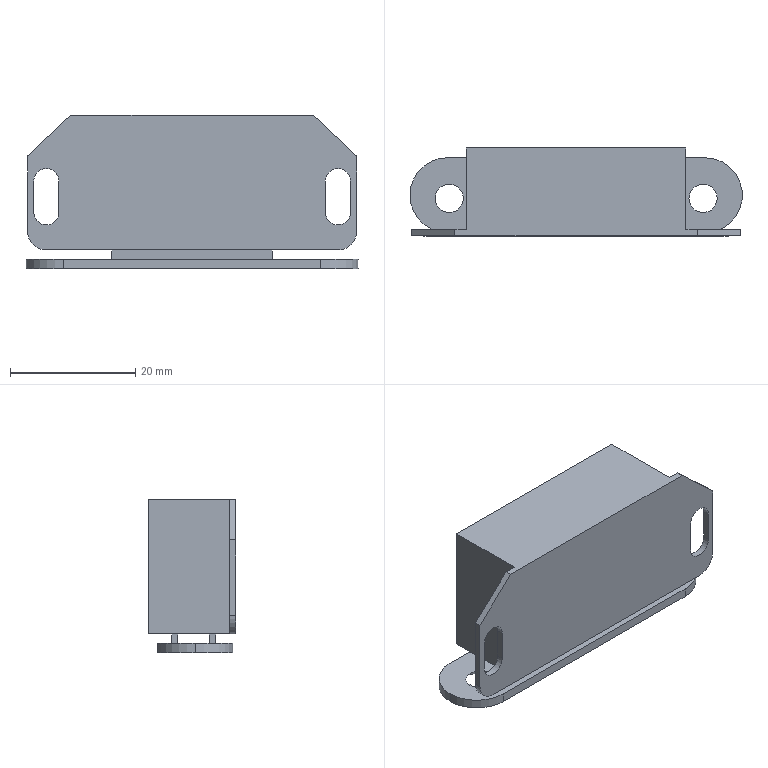Part | SolidWorks | features BaseBody 1 | 1 solid | 43 faces | box 53 x 14 x 24.5 mm | volume 11695 mm3 | plane 28 | cylinder 11 | cone 4 | commonest cylinder face diameters 4 x6 12 x3 6 x2
STEP:
#1=CARTESIAN_POINT('',(-21.25,0.,-10.5));
#2=VERTEX_POINT('',#1);
#3=CARTESIAN_POINT('',(-23.25,0.,-8.5));
#4=VERTEX_POINT('',#3);
#5=CARTESIAN_POINT('',(-23.25,0.,-10.5));
#6=DIRECTION('',(0.,-1.,0.));
#7=DIRECTION('',(0.,0.,1.));
#8=AXIS2_PLACEMENT_3D('',#5,#6,#7);
#9=CIRCLE('',#8,2.);
#10=EDGE_CURVE('',#2,#4,#9,.T.);
#11=ORIENTED_EDGE('',*,*,#10,.T.);
#12=CARTESIAN_POINT('',(-23.25,1.,-8.5));
#13=VERTEX_POINT('',#12);
#14=CARTESIAN_POINT('',(-23.25,1.,-8.5));
#15=DIRECTION('',(0.,1.,0.));
#16=VECTOR('',#15,1000.);
#17=LINE('',#14,#16);
#18=EDGE_CURVE('',#4,#13,#17,.T.);
#19=ORIENTED_EDGE('',*,*,#18,.T.);
#20=CARTESIAN_POINT('',(-21.25,1.,-10.5));
#21=VERTEX_POINT('',#20);
#22=CARTESIAN_POINT('',(-23.25,1.,-10.5));
#23=DIRECTION('',(0.,-1.,0.));
#24=DIRECTION('',(0.,0.,1.));
#25=AXIS2_PLACEMENT_3D('',#22,#23,#24);
#26=CIRCLE('',#25,2.);
#27=EDGE_CURVE('',#21,#13,#26,.T.);
#28=ORIENTED_EDGE('',*,*,#27,.F.);
#29=CARTESIAN_POINT('',(-21.25,1.,-10.5));
#30=DIRECTION('',(0.,1.,0.));
#31=VECTOR('',#30,1000.);
#32=LINE('',#29,#31);
#33=EDGE_CURVE('',#2,#21,#32,.T.);
#34=ORIENTED_EDGE('',*,*,#33,.F.);
#35=EDGE_LOOP('',(#11,#19,#28,#34));
#36=FACE_OUTER_BOUND('',#35,.T.);
#37=CARTESIAN_POINT('',(-23.25,1.,-10.5));
#38=DIRECTION('',(0.,1.,0.));
#39=DIRECTION('',(0.,0.,1.));
#40=AXIS2_PLACEMENT_3D('',#37,#38,#39);
#41=CYLINDRICAL_SURFACE('',#40,2.);
#42=ADVANCED_FACE('',(#36),#41,.F.);
#43=CARTESIAN_POINT('',(25.25,0.,-10.5));
#44=VERTEX_POINT('',#43);
#45=CARTESIAN_POINT('',(23.25,0.,-8.5));
#46=VERTEX_POINT('',#45);
#47=CARTESIAN_POINT('',(23.25,0.,-10.5));
#48=DIRECTION('',(0.,-1.,0.));
#49=DIRECTION('',(0.,0.,1.));
#50=AXIS2_PLACEMENT_3D('',#47,#48,#49);
#51=CIRCLE('',#50,2.);
#52=EDGE_CURVE('',#44,#46,#51,.T.);
#53=ORIENTED_EDGE('',*,*,#52,.T.);
#54=CARTESIAN_POINT('',(23.25,1.,-8.5));
#55=VERTEX_POINT('',#54);
#56=CARTESIAN_POINT('',(23.25,1.,-8.5));
#57=DIRECTION('',(0.,1.,0.));
#58=VECTOR('',#57,1000.);
#59=LINE('',#56,#58);
#60=EDGE_CURVE('',#46,#55,#59,.T.);
#61=ORIENTED_EDGE('',*,*,#60,.T.);
#62=CARTESIAN_POINT('',(25.25,1.,-10.5));
#63=VERTEX_POINT('',#62);
#64=CARTESIAN_POINT('',(23.25,1.,-10.5));
#65=DIRECTION('',(0.,-1.,0.));
#66=DIRECTION('',(0.,0.,1.));
#67=AXIS2_PLACEMENT_3D('',#64,#65,#66);
#68=CIRCLE('',#67,2.);
#69=EDGE_CURVE('',#63,#55,#68,.T.);
#70=ORIENTED_EDGE('',*,*,#69,.F.);
#71=CARTESIAN_POINT('',(25.25,1.,-10.5));
#72=DIRECTION('',(0.,1.,0.));
#73=VECTOR('',#72,1000.);
#74=LINE('',#71,#73);
#75=EDGE_CURVE('',#44,#63,#74,.T.);
#76=ORIENTED_EDGE('',*,*,#75,.F.);
#77=EDGE_LOOP('',(#53,#61,#70,#76));
#78=FACE_OUTER_BOUND('',#77,.T.);
#79=CARTESIAN_POINT('',(23.25,1.,-10.5));
#80=DIRECTION('',(0.,1.,0.));
#81=DIRECTION('',(0.,0.,1.));
#82=AXIS2_PLACEMENT_3D('',#79,#80,#81);
#83=CYLINDRICAL_SURFACE('',#82,2.);
#84=ADVANCED_FACE('',(#78),#83,.F.);
#85=CARTESIAN_POINT('',(-26.5,6.5,-23.));
#86=VERTEX_POINT('',#85);
#87=CARTESIAN_POINT('',(-20.5,0.5,-23.));
#88=VERTEX_POINT('',#87);
#89=CARTESIAN_POINT('',(-20.5,6.5,-23.));
#90=DIRECTION('',(0.,0.,1.));
#91=DIRECTION('',(-1.,0.,0.));
#92=AXIS2_PLACEMENT_3D('',#89,#90,#91);
#93=CIRCLE('',#92,6.);
#94=EDGE_CURVE('',#86,#88,#93,.T.);
#95=ORIENTED_EDGE('',*,*,#94,.F.);
#96=CARTESIAN_POINT('',(-26.5,6.5,-24.5));
#97=VERTEX_POINT('',#96);
#98=CARTESIAN_POINT('',(-26.5,6.5,-24.5));
#99=DIRECTION('',(0.,0.,-1.));
#100=VECTOR('',#99,1000.);
#101=LINE('',#98,#100);
#102=EDGE_CURVE('',#86,#97,#101,.T.);
#103=ORIENTED_EDGE('',*,*,#102,.T.);
#104=CARTESIAN_POINT('',(-20.5,0.5,-24.5));
#105=VERTEX_POINT('',#104);
#106=CARTESIAN_POINT('',(-20.5,6.5,-24.5));
#107=DIRECTION('',(0.,0.,1.));
#108=DIRECTION('',(-1.,0.,0.));
#109=AXIS2_PLACEMENT_3D('',#106,#107,#108);
#110=CIRCLE('',#109,6.);
#111=EDGE_CURVE('',#97,#105,#110,.T.);
#112=ORIENTED_EDGE('',*,*,#111,.T.);
#113=CARTESIAN_POINT('',(-20.5,0.5,-24.5));
#114=DIRECTION('',(0.,0.,-1.));
#115=VECTOR('',#114,1000.);
#116=LINE('',#113,#115);
#117=EDGE_CURVE('',#88,#105,#116,.T.);
#118=ORIENTED_EDGE('',*,*,#117,.F.);
#119=EDGE_LOOP('',(#95,#103,#112,#118));
#120=FACE_OUTER_BOUND('',#119,.T.);
#121=CARTESIAN_POINT('',(-20.5,6.5,-24.5));
#122=DIRECTION('',(0.,0.,-1.));
#123=DIRECTION('',(-1.,0.,0.));
#124=AXIS2_PLACEMENT_3D('',#121,#122,#123);
#125=CYLINDRICAL_SURFACE('',#124,6.);
#126=ADVANCED_FACE('',(#120),#125,.T.);
#127=CARTESIAN_POINT('',(-18.,6.,-23.));
#128=VERTEX_POINT('',#127);
#129=CARTESIAN_POINT('',(-22.5,6.,-23.));
#130=VERTEX_POINT('',#129);
#131=CARTESIAN_POINT('',(-20.25,6.,-23.));
#132=DIRECTION('',(0.,0.,-1.));
#133=DIRECTION('',(-1.,0.,0.));
#134=AXIS2_PLACEMENT_3D('',#131,#132,#133);
#135=CIRCLE('',#134,2.25);
#136=EDGE_CURVE('',#128,#130,#135,.T.);
#137=ORIENTED_EDGE('',*,*,#136,.F.);
#138=CARTESIAN_POINT('',(-16.5,6.,-24.5));
#139=VERTEX_POINT('',#138);
#140=CARTESIAN_POINT('',(-16.5,6.,-24.5));
#141=DIRECTION('',(0.7071,0.,-0.7071));
#142=VECTOR('',#141,1000.);
#143=LINE('',#140,#142);
#144=EDGE_CURVE('',#128,#139,#143,.T.);
#145=ORIENTED_EDGE('',*,*,#144,.T.);
#146=CARTESIAN_POINT('',(-24.,6.,-24.5));
#147=VERTEX_POINT('',#146);
#148=CARTESIAN_POINT('',(-20.25,6.,-24.5));
#149=DIRECTION('',(0.,0.,1.));
#150=DIRECTION('',(-1.,0.,0.));
#151=AXIS2_PLACEMENT_3D('',#148,#149,#150);
#152=CIRCLE('',#151,3.75);
#153=EDGE_CURVE('',#147,#139,#152,.T.);
#154=ORIENTED_EDGE('',*,*,#153,.F.);
#155=CARTESIAN_POINT('',(-24.,6.,-24.5));
#156=DIRECTION('',(-0.7071,0.,-0.7071));
#157=VECTOR('',#156,1000.);
#158=LINE('',#155,#157);
#159=EDGE_CURVE('',#130,#147,#158,.T.);
#160=ORIENTED_EDGE('',*,*,#159,.F.);
#161=EDGE_LOOP('',(#137,#145,#154,#160));
#162=FACE_OUTER_BOUND('',#161,.T.);
#163=CARTESIAN_POINT('',(-20.25,6.,-24.5));
#164=DIRECTION('',(0.,0.,-1.));
#165=DIRECTION('',(-1.,0.,0.));
#166=AXIS2_PLACEMENT_3D('',#163,#164,#165);
#167=CONICAL_SURFACE('',#166,3.75,0.7854);
#168=ADVANCED_FACE('',(#162),#167,.F.);
#169=CARTESIAN_POINT('',(22.5,6.,-23.));
#170=VERTEX_POINT('',#169);
#171=CARTESIAN_POINT('',(18.,6.,-23.));
#172=VERTEX_POINT('',#171);
#173=CARTESIAN_POINT('',(20.25,6.,-23.));
#174=DIRECTION('',(0.,0.,-1.));
#175=DIRECTION('',(-1.,0.,0.));
#176=AXIS2_PLACEMENT_3D('',#173,#174,#175);
#177=CIRCLE('',#176,2.25);
#178=EDGE_CURVE('',#170,#172,#177,.T.);
#179=ORIENTED_EDGE('',*,*,#178,.F.);
#180=CARTESIAN_POINT('',(24.,6.,-24.5));
#181=VERTEX_POINT('',#180);
#182=CARTESIAN_POINT('',(24.,6.,-24.5));
#183=DIRECTION('',(0.7071,0.,-0.7071));
#184=VECTOR('',#183,1000.);
#185=LINE('',#182,#184);
#186=EDGE_CURVE('',#170,#181,#185,.T.);
#187=ORIENTED_EDGE('',*,*,#186,.T.);
#188=CARTESIAN_POINT('',(16.5,6.,-24.5));
#189=VERTEX_POINT('',#188);
#190=CARTESIAN_POINT('',(20.25,6.,-24.5));
#191=DIRECTION('',(0.,0.,1.));
#192=DIRECTION('',(-1.,0.,0.));
#193=AXIS2_PLACEMENT_3D('',#190,#191,#192);
#194=CIRCLE('',#193,3.75);
#195=EDGE_CURVE('',#189,#181,#194,.T.);
#196=ORIENTED_EDGE('',*,*,#195,.F.);
#197=CARTESIAN_POINT('',(16.5,6.,-24.5));
#198=DIRECTION('',(-0.7071,0.,-0.7071));
#199=VECTOR('',#198,1000.);
#200=LINE('',#197,#199);
#201=EDGE_CURVE('',#172,#189,#200,.T.);
#202=ORIENTED_EDGE('',*,*,#201,.F.);
#203=EDGE_LOOP('',(#179,#187,#196,#202));
#204=FACE_OUTER_BOUND('',#203,.T.);
#205=CARTESIAN_POINT('',(20.25,6.,-24.5));
#206=DIRECTION('',(0.,0.,-1.));
#207=DIRECTION('',(-1.,0.,0.));
#208=AXIS2_PLACEMENT_3D('',#205,#206,#207);
#209=CONICAL_SURFACE('',#208,3.75,0.7854);
#210=ADVANCED_FACE('',(#204),#209,.F.);
#211=ORIENTED_EDGE('',*,*,#10,.F.);
#212=CARTESIAN_POINT('',(-21.25,0.,-15.5));
#213=VERTEX_POINT('',#212);
#214=CARTESIAN_POINT('',(-21.25,0.,-18.5));
#215=DIRECTION('',(0.,0.,1.));
#216=VECTOR('',#215,1000.);
#217=LINE('',#214,#216);
#218=EDGE_CURVE('',#213,#2,#217,.T.);
#219=ORIENTED_EDGE('',*,*,#218,.F.);
#220=CARTESIAN_POINT('',(-25.25,0.,-15.5));
#221=VERTEX_POINT('',#220);
#222=CARTESIAN_POINT('',(-23.25,0.,-15.5));
#223=DIRECTION('',(0.,-1.,0.));
#224=DIRECTION('',(0.,0.,1.));
#225=AXIS2_PLACEMENT_3D('',#222,#223,#224);
#226=CIRCLE('',#225,2.);
#227=EDGE_CURVE('',#221,#213,#226,.T.);
#228=ORIENTED_EDGE('',*,*,#227,.F.);
#229=CARTESIAN_POINT('',(-25.25,0.,-10.5));
#230=VERTEX_POINT('',#229);
#231=CARTESIAN_POINT('',(-25.25,0.,-18.5));
#232=DIRECTION('',(0.,0.,-1.));
#233=VECTOR('',#232,1000.);
#234=LINE('',#231,#233);
#235=EDGE_CURVE('',#230,#221,#234,.T.);
#236=ORIENTED_EDGE('',*,*,#235,.F.);
#237=CARTESIAN_POINT('',(-23.25,0.,-10.5));
#238=DIRECTION('',(0.,-1.,0.));
#239=DIRECTION('',(0.,0.,1.));
#240=AXIS2_PLACEMENT_3D('',#237,#238,#239);
#241=CIRCLE('',#240,2.);
#242=EDGE_CURVE('',#4,#230,#241,.T.);
#243=ORIENTED_EDGE('',*,*,#242,.F.);
#244=EDGE_LOOP('',(#211,#219,#228,#236,#243));
#245=FACE_BOUND('',#244,.T.);
#246=ORIENTED_EDGE('',*,*,#52,.F.);
#247=CARTESIAN_POINT('',(25.25,0.,-15.5));
#248=VERTEX_POINT('',#247);
#249=CARTESIAN_POINT('',(25.25,0.,-18.5));
#250=DIRECTION('',(0.,0.,1.));
#251=VECTOR('',#250,1000.);
#252=LINE('',#249,#251);
#253=EDGE_CURVE('',#248,#44,#252,.T.);
#254=ORIENTED_EDGE('',*,*,#253,.F.);
#255=CARTESIAN_POINT('',(21.25,0.,-15.5));
#256=VERTEX_POINT('',#255);
#257=CARTESIAN_POINT('',(23.25,0.,-15.5));
#258=DIRECTION('',(0.,-1.,0.));
#259=DIRECTION('',(0.,0.,1.));
#260=AXIS2_PLACEMENT_3D('',#257,#258,#259);
#261=CIRCLE('',#260,2.);
#262=EDGE_CURVE('',#256,#248,#261,.T.);
#263=ORIENTED_EDGE('',*,*,#262,.F.);
#264=CARTESIAN_POINT('',(21.25,0.,-10.5));
#265=VERTEX_POINT('',#264);
#266=CARTESIAN_POINT('',(21.25,0.,-18.5));
#267=DIRECTION('',(0.,0.,-1.));
#268=VECTOR('',#267,1000.);
#269=LINE('',#266,#268);
#270=EDGE_CURVE('',#265,#256,#269,.T.);
#271=ORIENTED_EDGE('',*,*,#270,.F.);
#272=CARTESIAN_POINT('',(23.25,0.,-10.5));
#273=DIRECTION('',(0.,-1.,0.));
#274=DIRECTION('',(0.,0.,1.));
#275=AXIS2_PLACEMENT_3D('',#272,#273,#274);
#276=CIRCLE('',#275,2.);
#277=EDGE_CURVE('',#46,#265,#276,.T.);
#278=ORIENTED_EDGE('',*,*,#277,.F.);
#279=EDGE_LOOP('',(#246,#254,#263,#271,#278));
#280=FACE_BOUND('',#279,.T.);
#281=CARTESIAN_POINT('',(-19.344,0.,0.));
#282=VERTEX_POINT('',#281);
#283=CARTESIAN_POINT('',(19.344,0.,0.));
#284=VERTEX_POINT('',#283);
#285=CARTESIAN_POINT('',(23.25,0.,0.));
#286=DIRECTION('',(1.,0.,0.));
#287=VECTOR('',#286,1000.);
#288=LINE('',#285,#287);
#289=EDGE_CURVE('',#282,#284,#288,.T.);
#290=ORIENTED_EDGE('',*,*,#289,.F.);
#291=CARTESIAN_POINT('',(-26.25,0.,-6.5));
#292=VERTEX_POINT('',#291);
#293=CARTESIAN_POINT('',(-26.25,0.,-6.5));
#294=DIRECTION('',(0.7282,0.,0.6854));
#295=VECTOR('',#294,1000.);
#296=LINE('',#293,#295);
#297=EDGE_CURVE('',#292,#282,#296,.T.);
#298=ORIENTED_EDGE('',*,*,#297,.F.);
#299=CARTESIAN_POINT('',(-26.25,0.,-18.5));
#300=VERTEX_POINT('',#299);
#301=CARTESIAN_POINT('',(-26.25,0.,-18.5));
#302=DIRECTION('',(0.,0.,1.));
#303=VECTOR('',#302,1000.);
#304=LINE('',#301,#303);
#305=EDGE_CURVE('',#300,#292,#304,.T.);
#306=ORIENTED_EDGE('',*,*,#305,.F.);
#307=CARTESIAN_POINT('',(-23.25,0.,-21.5));
#308=VERTEX_POINT('',#307);
#309=CARTESIAN_POINT('',(-23.25,0.,-18.5));
#310=DIRECTION('',(0.,1.,0.));
#311=DIRECTION('',(0.,0.,1.));
#312=AXIS2_PLACEMENT_3D('',#309,#310,#311);
#313=CIRCLE('',#312,3.);
#314=EDGE_CURVE('',#308,#300,#313,.T.);
#315=ORIENTED_EDGE('',*,*,#314,.F.);
#316=CARTESIAN_POINT('',(23.25,0.,-21.5));
#317=VERTEX_POINT('',#316);
#318=CARTESIAN_POINT('',(23.25,0.,-21.5));
#319=DIRECTION('',(-1.,0.,0.));
#320=VECTOR('',#319,1000.);
#321=LINE('',#318,#320);
#322=EDGE_CURVE('',#317,#308,#321,.T.);
#323=ORIENTED_EDGE('',*,*,#322,.F.);
#324=CARTESIAN_POINT('',(26.25,0.,-18.5));
#325=VERTEX_POINT('',#324);
#326=CARTESIAN_POINT('',(23.25,0.,-18.5));
#327=DIRECTION('',(0.,1.,0.));
#328=DIRECTION('',(0.,0.,1.));
#329=AXIS2_PLACEMENT_3D('',#326,#327,#328);
#330=CIRCLE('',#329,3.);
#331=EDGE_CURVE('',#325,#317,#330,.T.);
#332=ORIENTED_EDGE('',*,*,#331,.F.);
#333=CARTESIAN_POINT('',(26.25,0.,-6.5));
#334=VERTEX_POINT('',#333);
#335=CARTESIAN_POINT('',(26.25,0.,-18.5));
#336=DIRECTION('',(0.,0.,-1.));
#337=VECTOR('',#336,1000.);
#338=LINE('',#335,#337);
#339=EDGE_CURVE('',#334,#325,#338,.T.);
#340=ORIENTED_EDGE('',*,*,#339,.F.);
#341=CARTESIAN_POINT('',(19.344,0.,0.));
#342=DIRECTION('',(0.7282,0.,-0.6854));
#343=VECTOR('',#342,1000.);
#344=LINE('',#341,#343);
#345=EDGE_CURVE('',#284,#334,#344,.T.);
#346=ORIENTED_EDGE('',*,*,#345,.F.);
#347=EDGE_LOOP('',(#290,#298,#306,#315,#323,#332,#340,#346));
#348=FACE_OUTER_BOUND('',#347,.T.);
#349=CARTESIAN_POINT('',(23.25,0.,-18.5));
#350=DIRECTION('',(0.,1.,0.));
#351=DIRECTION('',(0.,0.,1.));
#352=AXIS2_PLACEMENT_3D('',#349,#350,#351);
#353=PLANE('',#352);
#354=ADVANCED_FACE('',(#245,#280,#348),#353,.F.);
#355=CARTESIAN_POINT('',(-25.25,1.,-15.5));
#356=VERTEX_POINT('',#355);
#357=CARTESIAN_POINT('',(-25.25,1.,-10.5));
#358=VERTEX_POINT('',#357);
#359=CARTESIAN_POINT('',(-25.25,1.,-15.5));
#360=DIRECTION('',(0.,0.,1.));
#361=VECTOR('',#360,1000.);
#362=LINE('',#359,#361);
#363=EDGE_CURVE('',#356,#358,#362,.T.);
#364=ORIENTED_EDGE('',*,*,#363,.T.);
#365=CARTESIAN_POINT('',(-25.25,1.,-10.5));
#366=DIRECTION('',(0.,-1.,0.));
#367=VECTOR('',#366,1000.);
#368=LINE('',#365,#367);
#369=EDGE_CURVE('',#358,#230,#368,.T.);
#370=ORIENTED_EDGE('',*,*,#369,.T.);
#371=ORIENTED_EDGE('',*,*,#235,.T.);
#372=CARTESIAN_POINT('',(-25.25,1.,-15.5));
#373=DIRECTION('',(0.,1.,0.));
#374=VECTOR('',#373,1000.);
#375=LINE('',#372,#374);
#376=EDGE_CURVE('',#221,#356,#375,.T.);
#377=ORIENTED_EDGE('',*,*,#376,.T.);
#378=EDGE_LOOP('',(#364,#370,#371,#377));
#379=FACE_OUTER_BOUND('',#378,.T.);
#380=CARTESIAN_POINT('',(-25.25,1.,-15.5));
#381=DIRECTION('',(1.,0.,0.));
#382=DIRECTION('',(0.,0.,-1.));
#383=AXIS2_PLACEMENT_3D('',#380,#381,#382);
#384=PLANE('',#383);
#385=ADVANCED_FACE('',(#379),#384,.T.);
#386=ORIENTED_EDGE('',*,*,#18,.F.);
#387=ORIENTED_EDGE('',*,*,#242,.T.);
#388=ORIENTED_EDGE('',*,*,#369,.F.);
#389=CARTESIAN_POINT('',(-23.25,1.,-10.5));
#390=DIRECTION('',(0.,-1.,0.));
#391=DIRECTION('',(0.,0.,1.));
#392=AXIS2_PLACEMENT_3D('',#389,#390,#391);
#393=CIRCLE('',#392,2.);
#394=EDGE_CURVE('',#13,#358,#393,.T.);
#395=ORIENTED_EDGE('',*,*,#394,.F.);
#396=EDGE_LOOP('',(#386,#387,#388,#395));
#397=FACE_OUTER_BOUND('',#396,.T.);
#398=CARTESIAN_POINT('',(-23.25,1.,-10.5));
#399=DIRECTION('',(0.,1.,0.));
#400=DIRECTION('',(0.,0.,1.));
#401=AXIS2_PLACEMENT_3D('',#398,#399,#400);
#402=CYLINDRICAL_SURFACE('',#401,2.);
#403=ADVANCED_FACE('',(#397),#402,.F.);
#404=CARTESIAN_POINT('',(-21.25,1.,-15.5));
#405=VERTEX_POINT('',#404);
#406=CARTESIAN_POINT('',(-21.25,1.,-10.5));
#407=DIRECTION('',(0.,0.,-1.));
#408=VECTOR('',#407,1000.);
#409=LINE('',#406,#408);
#410=EDGE_CURVE('',#21,#405,#409,.T.);
#411=ORIENTED_EDGE('',*,*,#410,.T.);
#412=CARTESIAN_POINT('',(-21.25,1.,-15.5));
#413=DIRECTION('',(0.,-1.,0.));
#414=VECTOR('',#413,1000.);
#415=LINE('',#412,#414);
#416=EDGE_CURVE('',#405,#213,#415,.T.);
#417=ORIENTED_EDGE('',*,*,#416,.T.);
#418=ORIENTED_EDGE('',*,*,#218,.T.);
#419=ORIENTED_EDGE('',*,*,#33,.T.);
#420=EDGE_LOOP('',(#411,#417,#418,#419));
#421=FACE_OUTER_BOUND('',#420,.T.);
#422=CARTESIAN_POINT('',(-21.25,1.,-10.5));
#423=DIRECTION('',(-1.,0.,0.));
#424=DIRECTION('',(0.,0.,1.));
#425=AXIS2_PLACEMENT_3D('',#422,#423,#424);
#426=PLANE('',#425);
#427=ADVANCED_FACE('',(#421),#426,.T.);
#428=ORIENTED_EDGE('',*,*,#416,.F.);
#429=CARTESIAN_POINT('',(-23.25,1.,-15.5));
#430=DIRECTION('',(0.,-1.,0.));
#431=DIRECTION('',(0.,0.,1.));
#432=AXIS2_PLACEMENT_3D('',#429,#430,#431);
#433=CIRCLE('',#432,2.);
#434=EDGE_CURVE('',#356,#405,#433,.T.);
#435=ORIENTED_EDGE('',*,*,#434,.F.);
#436=ORIENTED_EDGE('',*,*,#376,.F.);
#437=ORIENTED_EDGE('',*,*,#227,.T.);
#438=EDGE_LOOP('',(#428,#435,#436,#437));
#439=FACE_OUTER_BOUND('',#438,.T.);
#440=CARTESIAN_POINT('',(-23.25,1.,-15.5));
#441=DIRECTION('',(0.,1.,0.));
#442=DIRECTION('',(0.,0.,1.));
#443=AXIS2_PLACEMENT_3D('',#440,#441,#442);
#444=CYLINDRICAL_SURFACE('',#443,2.);
#445=ADVANCED_FACE('',(#439),#444,.F.);
#446=CARTESIAN_POINT('',(21.25,1.,-15.5));
#447=VERTEX_POINT('',#446);
#448=CARTESIAN_POINT('',(21.25,1.,-10.5));
#449=VERTEX_POINT('',#448);
#450=CARTESIAN_POINT('',(21.25,1.,-15.5));
#451=DIRECTION('',(0.,0.,1.));
#452=VECTOR('',#451,1000.);
#453=LINE('',#450,#452);
#454=EDGE_CURVE('',#447,#449,#453,.T.);
#455=ORIENTED_EDGE('',*,*,#454,.T.);
#456=CARTESIAN_POINT('',(21.25,1.,-10.5));
#457=DIRECTION('',(0.,-1.,0.));
#458=VECTOR('',#457,1000.);
#459=LINE('',#456,#458);
#460=EDGE_CURVE('',#449,#265,#459,.T.);
#461=ORIENTED_EDGE('',*,*,#460,.T.);
#462=ORIENTED_EDGE('',*,*,#270,.T.);
#463=CARTESIAN_POINT('',(21.25,1.,-15.5));
#464=DIRECTION('',(0.,1.,0.));
#465=VECTOR('',#464,1000.);
#466=LINE('',#463,#465);
#467=EDGE_CURVE('',#256,#447,#466,.T.);
#468=ORIENTED_EDGE('',*,*,#467,.T.);
#469=EDGE_LOOP('',(#455,#461,#462,#468));
#470=FACE_OUTER_BOUND('',#469,.T.);
#471=CARTESIAN_POINT('',(21.25,1.,-15.5));
#472=DIRECTION('',(1.,0.,0.));
#473=DIRECTION('',(0.,0.,-1.));
#474=AXIS2_PLACEMENT_3D('',#471,#472,#473);
#475=PLANE('',#474);
#476=ADVANCED_FACE('',(#470),#475,.T.);
#477=ORIENTED_EDGE('',*,*,#60,.F.);
#478=ORIENTED_EDGE('',*,*,#277,.T.);
#479=ORIENTED_EDGE('',*,*,#460,.F.);
#480=CARTESIAN_POINT('',(23.25,1.,-10.5));
#481=DIRECTION('',(0.,-1.,0.));
#482=DIRECTION('',(0.,0.,1.));
#483=AXIS2_PLACEMENT_3D('',#480,#481,#482);
#484=CIRCLE('',#483,2.);
#485=EDGE_CURVE('',#55,#449,#484,.T.);
#486=ORIENTED_EDGE('',*,*,#485,.F.);
#487=EDGE_LOOP('',(#477,#478,#479,#486));
#488=FACE_OUTER_BOUND('',#487,.T.);
#489=CARTESIAN_POINT('',(23.25,1.,-10.5));
#490=DIRECTION('',(0.,1.,0.));
#491=DIRECTION('',(0.,0.,1.));
#492=AXIS2_PLACEMENT_3D('',#489,#490,#491);
#493=CYLINDRICAL_SURFACE('',#492,2.);
#494=ADVANCED_FACE('',(#488),#493,.F.);
#495=CARTESIAN_POINT('',(25.25,1.,-15.5));
#496=VERTEX_POINT('',#495);
#497=CARTESIAN_POINT('',(25.25,1.,-10.5));
#498=DIRECTION('',(0.,0.,-1.));
#499=VECTOR('',#498,1000.);
#500=LINE('',#497,#499);
#501=EDGE_CURVE('',#63,#496,#500,.T.);
#502=ORIENTED_EDGE('',*,*,#501,.T.);
#503=CARTESIAN_POINT('',(25.25,1.,-15.5));
#504=DIRECTION('',(0.,-1.,0.));
#505=VECTOR('',#504,1000.);
#506=LINE('',#503,#505);
#507=EDGE_CURVE('',#496,#248,#506,.T.);
#508=ORIENTED_EDGE('',*,*,#507,.T.);
#509=ORIENTED_EDGE('',*,*,#253,.T.);
#510=ORIENTED_EDGE('',*,*,#75,.T.);
#511=EDGE_LOOP('',(#502,#508,#509,#510));
#512=FACE_OUTER_BOUND('',#511,.T.);
#513=CARTESIAN_POINT('',(25.25,1.,-10.5));
#514=DIRECTION('',(-1.,0.,0.));
#515=DIRECTION('',(0.,0.,1.));
#516=AXIS2_PLACEMENT_3D('',#513,#514,#515);
#517=PLANE('',#516);
#518=ADVANCED_FACE('',(#512),#517,.T.);
#519=ORIENTED_EDGE('',*,*,#507,.F.);
#520=CARTESIAN_POINT('',(23.25,1.,-15.5));
#521=DIRECTION('',(0.,-1.,0.));
#522=DIRECTION('',(0.,0.,1.));
#523=AXIS2_PLACEMENT_3D('',#520,#521,#522);
#524=CIRCLE('',#523,2.);
#525=EDGE_CURVE('',#447,#496,#524,.T.);
#526=ORIENTED_EDGE('',*,*,#525,.F.);
#527=ORIENTED_EDGE('',*,*,#467,.F.);
#528=ORIENTED_EDGE('',*,*,#262,.T.);
#529=EDGE_LOOP('',(#519,#526,#527,#528));
#530=FACE_OUTER_BOUND('',#529,.T.);
#531=CARTESIAN_POINT('',(23.25,1.,-15.5));
#532=DIRECTION('',(0.,1.,0.));
#533=DIRECTION('',(0.,0.,1.));
#534=AXIS2_PLACEMENT_3D('',#531,#532,#533);
#535=CYLINDRICAL_SURFACE('',#534,2.);
#536=ADVANCED_FACE('',(#530),#535,.F.);
#537=CARTESIAN_POINT('',(26.25,1.,-6.5));
#538=VERTEX_POINT('',#537);
#539=CARTESIAN_POINT('',(26.25,1.,-6.5));
#540=DIRECTION('',(0.,-1.,0.));
#541=VECTOR('',#540,1000.);
#542=LINE('',#539,#541);
#543=EDGE_CURVE('',#538,#334,#542,.T.);
#544=ORIENTED_EDGE('',*,*,#543,.F.);
#545=CARTESIAN_POINT('',(19.344,1.,0.));
#546=VERTEX_POINT('',#545);
#547=CARTESIAN_POINT('',(19.344,1.,0.));
#548=DIRECTION('',(0.7282,0.,-0.6854));
#549=VECTOR('',#548,1000.);
#550=LINE('',#547,#549);
#551=EDGE_CURVE('',#546,#538,#550,.T.);
#552=ORIENTED_EDGE('',*,*,#551,.F.);
#553=CARTESIAN_POINT('',(19.344,1.,0.));
#554=DIRECTION('',(0.,1.,0.));
#555=VECTOR('',#554,1000.);
#556=LINE('',#553,#555);
#557=EDGE_CURVE('',#284,#546,#556,.T.);
#558=ORIENTED_EDGE('',*,*,#557,.F.);
#559=ORIENTED_EDGE('',*,*,#345,.T.);
#560=EDGE_LOOP('',(#544,#552,#558,#559));
#561=FACE_OUTER_BOUND('',#560,.T.);
#562=CARTESIAN_POINT('',(19.344,1.,0.));
#563=DIRECTION('',(-0.6854,0.,-0.7282));
#564=DIRECTION('',(-0.7282,0.,0.6854));
#565=AXIS2_PLACEMENT_3D('',#562,#563,#564);
#566=PLANE('',#565);
#567=ADVANCED_FACE('',(#561),#566,.F.);
#568=ORIENTED_EDGE('',*,*,#557,.T.);
#569=CARTESIAN_POINT('',(17.5,1.,0.));
#570=VERTEX_POINT('',#569);
#571=CARTESIAN_POINT('',(-19.344,1.,0.));
#572=DIRECTION('',(1.,0.,0.));
#573=VECTOR('',#572,1000.);
#574=LINE('',#571,#573);
#575=EDGE_CURVE('',#570,#546,#574,.T.);
#576=ORIENTED_EDGE('',*,*,#575,.F.);
#577=CARTESIAN_POINT('',(17.5,14.,0.));
#578=VERTEX_POINT('',#577);
#579=CARTESIAN_POINT('',(17.5,1.,0.));
#580=DIRECTION('',(0.,-1.,0.));
#581=VECTOR('',#580,1000.);
#582=LINE('',#579,#581);
#583=EDGE_CURVE('',#578,#570,#582,.T.);
#584=ORIENTED_EDGE('',*,*,#583,.F.);
#585=CARTESIAN_POINT('',(-17.5,14.,0.));
#586=VERTEX_POINT('',#585);
#587=CARTESIAN_POINT('',(-19.344,14.,0.));
#588=DIRECTION('',(1.,0.,0.));
#589=VECTOR('',#588,1000.);
#590=LINE('',#587,#589);
#591=EDGE_CURVE('',#586,#578,#590,.T.);
#592=ORIENTED_EDGE('',*,*,#591,.F.);
#593=CARTESIAN_POINT('',(-17.5,1.,0.));
#594=VERTEX_POINT('',#593);
#595=CARTESIAN_POINT('',(-17.5,1.,0.));
#596=DIRECTION('',(0.,1.,0.));
#597=VECTOR('',#596,1000.);
#598=LINE('',#595,#597);
#599=EDGE_CURVE('',#594,#586,#598,.T.);
#600=ORIENTED_EDGE('',*,*,#599,.F.);
#601=CARTESIAN_POINT('',(-19.344,1.,0.));
#602=VERTEX_POINT('',#601);
#603=CARTESIAN_POINT('',(-19.344,1.,0.));
#604=DIRECTION('',(1.,0.,0.));
#605=VECTOR('',#604,1000.);
#606=LINE('',#603,#605);
#607=EDGE_CURVE('',#602,#594,#606,.T.);
#608=ORIENTED_EDGE('',*,*,#607,.F.);
#609=CARTESIAN_POINT('',(-19.344,1.,0.));
#610=DIRECTION('',(0.,1.,0.));
#611=VECTOR('',#610,1000.);
#612=LINE('',#609,#611);
#613=EDGE_CURVE('',#282,#602,#612,.T.);
#614=ORIENTED_EDGE('',*,*,#613,.F.);
#615=ORIENTED_EDGE('',*,*,#289,.T.);
#616=EDGE_LOOP('',(#568,#576,#584,#592,#600,#608,#614,#615));
#617=FACE_OUTER_BOUND('',#616,.T.);
#618=CARTESIAN_POINT('',(-19.344,1.,0.));
#619=DIRECTION('',(0.,0.,-1.));
#620=DIRECTION('',(-1.,0.,0.));
#621=AXIS2_PLACEMENT_3D('',#618,#619,#620);
#622=PLANE('',#621);
#623=ADVANCED_FACE('',(#617),#622,.F.);
#624=ORIENTED_EDGE('',*,*,#613,.T.);
#625=CARTESIAN_POINT('',(-26.25,1.,-6.5));
#626=VERTEX_POINT('',#625);
#627=CARTESIAN_POINT('',(-26.25,1.,-6.5));
#628=DIRECTION('',(0.7282,0.,0.6854));
#629=VECTOR('',#628,1000.);
#630=LINE('',#627,#629);
#631=EDGE_CURVE('',#626,#602,#630,.T.);
#632=ORIENTED_EDGE('',*,*,#631,.F.);
#633=CARTESIAN_POINT('',(-26.25,1.,-6.5));
#634=DIRECTION('',(0.,1.,0.));
#635=VECTOR('',#634,1000.);
#636=LINE('',#633,#635);
#637=EDGE_CURVE('',#292,#626,#636,.T.);
#638=ORIENTED_EDGE('',*,*,#637,.F.);
#639=ORIENTED_EDGE('',*,*,#297,.T.);
#640=EDGE_LOOP('',(#624,#632,#638,#639));
#641=FACE_OUTER_BOUND('',#640,.T.);
#642=CARTESIAN_POINT('',(-26.25,1.,-6.5));
#643=DIRECTION('',(0.6854,0.,-0.7282));
#644=DIRECTION('',(-0.7282,0.,-0.6854));
#645=AXIS2_PLACEMENT_3D('',#642,#643,#644);
#646=PLANE('',#645);
#647=ADVANCED_FACE('',(#641),#646,.F.);
#648=ORIENTED_EDGE('',*,*,#637,.T.);
#649=CARTESIAN_POINT('',(-26.25,1.,-18.5));
#650=VERTEX_POINT('',#649);
#651=CARTESIAN_POINT('',(-26.25,1.,-18.5));
#652=DIRECTION('',(0.,0.,1.));
#653=VECTOR('',#652,1000.);
#654=LINE('',#651,#653);
#655=EDGE_CURVE('',#650,#626,#654,.T.);
#656=ORIENTED_EDGE('',*,*,#655,.F.);
#657=CARTESIAN_POINT('',(-26.25,1.,-18.5));
#658=DIRECTION('',(0.,1.,0.));
#659=VECTOR('',#658,1000.);
#660=LINE('',#657,#659);
#661=EDGE_CURVE('',#300,#650,#660,.T.);
#662=ORIENTED_EDGE('',*,*,#661,.F.);
#663=ORIENTED_EDGE('',*,*,#305,.T.);
#664=EDGE_LOOP('',(#648,#656,#662,#663));
#665=FACE_OUTER_BOUND('',#664,.T.);
#666=CARTESIAN_POINT('',(-26.25,1.,-18.5));
#667=DIRECTION('',(1.,0.,0.));
#668=DIRECTION('',(0.,0.,-1.));
#669=AXIS2_PLACEMENT_3D('',#666,#667,#668);
#670=PLANE('',#669);
#671=ADVANCED_FACE('',(#665),#670,.F.);
#672=CARTESIAN_POINT('',(-23.25,1.,-21.5));
#673=VERTEX_POINT('',#672);
#674=CARTESIAN_POINT('',(-23.25,1.,-18.5));
#675=DIRECTION('',(0.,-1.,0.));
#676=DIRECTION('',(0.,0.,1.));
#677=AXIS2_PLACEMENT_3D('',#674,#675,#676);
#678=CIRCLE('',#677,3.);
#679=EDGE_CURVE('',#650,#673,#678,.T.);
#680=ORIENTED_EDGE('',*,*,#679,.T.);
#681=CARTESIAN_POINT('',(-23.25,1.,-21.5));
#682=DIRECTION('',(0.,-1.,0.));
#683=VECTOR('',#682,1000.);
#684=LINE('',#681,#683);
#685=EDGE_CURVE('',#673,#308,#684,.T.);
#686=ORIENTED_EDGE('',*,*,#685,.T.);
#687=ORIENTED_EDGE('',*,*,#314,.T.);
#688=ORIENTED_EDGE('',*,*,#661,.T.);
#689=EDGE_LOOP('',(#680,#686,#687,#688));
#690=FACE_OUTER_BOUND('',#689,.T.);
#691=CARTESIAN_POINT('',(-23.25,1.,-18.5));
#692=DIRECTION('',(0.,1.,0.));
#693=DIRECTION('',(0.,0.,1.));
#694=AXIS2_PLACEMENT_3D('',#691,#692,#693);
#695=CYLINDRICAL_SURFACE('',#694,3.);
#696=ADVANCED_FACE('',(#690),#695,.T.);
#697=ORIENTED_EDGE('',*,*,#685,.F.);
#698=CARTESIAN_POINT('',(-17.5,1.,-21.5));
#699=VERTEX_POINT('',#698);
#700=CARTESIAN_POINT('',(23.25,1.,-21.5));
#701=DIRECTION('',(-1.,0.,0.));
#702=VECTOR('',#701,1000.);
#703=LINE('',#700,#702);
#704=EDGE_CURVE('',#699,#673,#703,.T.);
#705=ORIENTED_EDGE('',*,*,#704,.F.);
#706=CARTESIAN_POINT('',(-17.5,14.,-21.5));
#707=VERTEX_POINT('',#706);
#708=CARTESIAN_POINT('',(-17.5,1.,-21.5));
#709=DIRECTION('',(0.,-1.,0.));
#710=VECTOR('',#709,1000.);
#711=LINE('',#708,#710);
#712=EDGE_CURVE('',#707,#699,#711,.T.);
#713=ORIENTED_EDGE('',*,*,#712,.F.);
#714=CARTESIAN_POINT('',(17.5,14.,-21.5));
#715=VERTEX_POINT('',#714);
#716=CARTESIAN_POINT('',(23.25,14.,-21.5));
#717=DIRECTION('',(-1.,0.,0.));
#718=VECTOR('',#717,1000.);
#719=LINE('',#716,#718);
#720=EDGE_CURVE('',#715,#707,#719,.T.);
#721=ORIENTED_EDGE('',*,*,#720,.F.);
#722=CARTESIAN_POINT('',(17.5,1.,-21.5));
#723=VERTEX_POINT('',#722);
#724=CARTESIAN_POINT('',(17.5,1.,-21.5));
#725=DIRECTION('',(0.,1.,0.));
#726=VECTOR('',#725,1000.);
#727=LINE('',#724,#726);
#728=EDGE_CURVE('',#723,#715,#727,.T.);
#729=ORIENTED_EDGE('',*,*,#728,.F.);
#730=CARTESIAN_POINT('',(23.25,1.,-21.5));
#731=VERTEX_POINT('',#730);
#732=CARTESIAN_POINT('',(23.25,1.,-21.5));
#733=DIRECTION('',(-1.,0.,0.));
#734=VECTOR('',#733,1000.);
#735=LINE('',#732,#734);
#736=EDGE_CURVE('',#731,#723,#735,.T.);
#737=ORIENTED_EDGE('',*,*,#736,.F.);
#738=CARTESIAN_POINT('',(23.25,1.,-21.5));
#739=DIRECTION('',(0.,1.,0.));
#740=VECTOR('',#739,1000.);
#741=LINE('',#738,#740);
#742=EDGE_CURVE('',#317,#731,#741,.T.);
#743=ORIENTED_EDGE('',*,*,#742,.F.);
#744=ORIENTED_EDGE('',*,*,#322,.T.);
#745=EDGE_LOOP('',(#697,#705,#713,#721,#729,#737,#743,#744));
#746=FACE_OUTER_BOUND('',#745,.T.);
#747=CARTESIAN_POINT('',(12.8,4.25,-21.5));
#748=VERTEX_POINT('',#747);
#749=CARTESIAN_POINT('',(12.8,3.25,-21.5));
#750=VERTEX_POINT('',#749);
#751=CARTESIAN_POINT('',(12.8,1.,-21.5));
#752=DIRECTION('',(0.,-1.,0.));
#753=VECTOR('',#752,1000.);
#754=LINE('',#751,#753);
#755=EDGE_CURVE('',#748,#750,#754,.T.);
#756=ORIENTED_EDGE('',*,*,#755,.F.);
#757=CARTESIAN_POINT('',(-12.8,4.25,-21.5));
#758=VERTEX_POINT('',#757);
#759=CARTESIAN_POINT('',(23.25,4.25,-21.5));
#760=DIRECTION('',(1.,0.,0.));
#761=VECTOR('',#760,1000.);
#762=LINE('',#759,#761);
#763=EDGE_CURVE('',#758,#748,#762,.T.);
#764=ORIENTED_EDGE('',*,*,#763,.F.);
#765=CARTESIAN_POINT('',(-12.8,3.25,-21.5));
#766=VERTEX_POINT('',#765);
#767=CARTESIAN_POINT('',(-12.8,1.,-21.5));
#768=DIRECTION('',(0.,1.,0.));
#769=VECTOR('',#768,1000.);
#770=LINE('',#767,#769);
#771=EDGE_CURVE('',#766,#758,#770,.T.);
#772=ORIENTED_EDGE('',*,*,#771,.F.);
#773=CARTESIAN_POINT('',(23.25,3.25,-21.5));
#774=DIRECTION('',(-1.,0.,0.));
#775=VECTOR('',#774,1000.);
#776=LINE('',#773,#775);
#777=EDGE_CURVE('',#750,#766,#776,.T.);
#778=ORIENTED_EDGE('',*,*,#777,.F.);
#779=EDGE_LOOP('',(#756,#764,#772,#778));
#780=FACE_BOUND('',#779,.T.);
#781=CARTESIAN_POINT('',(12.8,10.25,-21.5));
#782=VERTEX_POINT('',#781);
#783=CARTESIAN_POINT('',(12.8,9.25,-21.5));
#784=VERTEX_POINT('',#783);
#785=CARTESIAN_POINT('',(12.8,1.,-21.5));
#786=DIRECTION('',(0.,-1.,0.));
#787=VECTOR('',#786,1000.);
#788=LINE('',#785,#787);
#789=EDGE_CURVE('',#782,#784,#788,.T.);
#790=ORIENTED_EDGE('',*,*,#789,.F.);
#791=CARTESIAN_POINT('',(-12.8,10.25,-21.5));
#792=VERTEX_POINT('',#791);
#793=CARTESIAN_POINT('',(23.25,10.25,-21.5));
#794=DIRECTION('',(1.,0.,0.));
#795=VECTOR('',#794,1000.);
#796=LINE('',#793,#795);
#797=EDGE_CURVE('',#792,#782,#796,.T.);
#798=ORIENTED_EDGE('',*,*,#797,.F.);
#799=CARTESIAN_POINT('',(-12.8,9.25,-21.5));
#800=VERTEX_POINT('',#799);
#801=CARTESIAN_POINT('',(-12.8,1.,-21.5));
#802=DIRECTION('',(0.,1.,0.));
#803=VECTOR('',#802,1000.);
#804=LINE('',#801,#803);
#805=EDGE_CURVE('',#800,#792,#804,.T.);
#806=ORIENTED_EDGE('',*,*,#805,.F.);
#807=CARTESIAN_POINT('',(23.25,9.25,-21.5));
#808=DIRECTION('',(-1.,0.,0.));
#809=VECTOR('',#808,1000.);
#810=LINE('',#807,#809);
#811=EDGE_CURVE('',#784,#800,#810,.T.);
#812=ORIENTED_EDGE('',*,*,#811,.F.);
#813=EDGE_LOOP('',(#790,#798,#806,#812));
#814=FACE_BOUND('',#813,.T.);
#815=CARTESIAN_POINT('',(23.25,1.,-21.5));
#816=DIRECTION('',(0.,0.,1.));
#817=DIRECTION('',(1.,0.,0.));
#818=AXIS2_PLACEMENT_3D('',#815,#816,#817);
#819=PLANE('',#818);
#820=ADVANCED_FACE('',(#746,#780,#814),#819,.F.);
#821=CARTESIAN_POINT('',(26.25,1.,-18.5));
#822=VERTEX_POINT('',#821);
#823=CARTESIAN_POINT('',(23.25,1.,-18.5));
#824=DIRECTION('',(0.,-1.,0.));
#825=DIRECTION('',(0.,0.,1.));
#826=AXIS2_PLACEMENT_3D('',#823,#824,#825);
#827=CIRCLE('',#826,3.);
#828=EDGE_CURVE('',#731,#822,#827,.T.);
#829=ORIENTED_EDGE('',*,*,#828,.T.);
#830=CARTESIAN_POINT('',(26.25,1.,-18.5));
#831=DIRECTION('',(0.,-1.,0.));
#832=VECTOR('',#831,1000.);
#833=LINE('',#830,#832);
#834=EDGE_CURVE('',#822,#325,#833,.T.);
#835=ORIENTED_EDGE('',*,*,#834,.T.);
#836=ORIENTED_EDGE('',*,*,#331,.T.);
#837=ORIENTED_EDGE('',*,*,#742,.T.);
#838=EDGE_LOOP('',(#829,#835,#836,#837));
#839=FACE_OUTER_BOUND('',#838,.T.);
#840=CARTESIAN_POINT('',(23.25,1.,-18.5));
#841=DIRECTION('',(0.,1.,0.));
#842=DIRECTION('',(0.,0.,1.));
#843=AXIS2_PLACEMENT_3D('',#840,#841,#842);
#844=CYLINDRICAL_SURFACE('',#843,3.);
#845=ADVANCED_FACE('',(#839),#844,.T.);
#846=ORIENTED_EDGE('',*,*,#834,.F.);
#847=CARTESIAN_POINT('',(26.25,1.,-6.5));
#848=DIRECTION('',(0.,0.,-1.));
#849=VECTOR('',#848,1000.);
#850=LINE('',#847,#849);
#851=EDGE_CURVE('',#538,#822,#850,.T.);
#852=ORIENTED_EDGE('',*,*,#851,.F.);
#853=ORIENTED_EDGE('',*,*,#543,.T.);
#854=ORIENTED_EDGE('',*,*,#339,.T.);
#855=EDGE_LOOP('',(#846,#852,#853,#854));
#856=FACE_OUTER_BOUND('',#855,.T.);
#857=CARTESIAN_POINT('',(26.25,1.,-6.5));
#858=DIRECTION('',(-1.,0.,0.));
#859=DIRECTION('',(0.,0.,1.));
#860=AXIS2_PLACEMENT_3D('',#857,#858,#859);
#861=PLANE('',#860);
#862=ADVANCED_FACE('',(#856),#861,.F.);
#863=ORIENTED_EDGE('',*,*,#655,.T.);
#864=ORIENTED_EDGE('',*,*,#631,.T.);
#865=ORIENTED_EDGE('',*,*,#607,.T.);
#866=CARTESIAN_POINT('',(-17.5,1.,-18.5));
#867=DIRECTION('',(0.,0.,-1.));
#868=VECTOR('',#867,1000.);
#869=LINE('',#866,#868);
#870=EDGE_CURVE('',#594,#699,#869,.T.);
#871=ORIENTED_EDGE('',*,*,#870,.T.);
#872=ORIENTED_EDGE('',*,*,#704,.T.);
#873=ORIENTED_EDGE('',*,*,#679,.F.);
#874=EDGE_LOOP('',(#863,#864,#865,#871,#872,#873));
#875=FACE_OUTER_BOUND('',#874,.T.);
#876=ORIENTED_EDGE('',*,*,#410,.F.);
#877=ORIENTED_EDGE('',*,*,#27,.T.);
#878=ORIENTED_EDGE('',*,*,#394,.T.);
#879=ORIENTED_EDGE('',*,*,#363,.F.);
#880=ORIENTED_EDGE('',*,*,#434,.T.);
#881=EDGE_LOOP('',(#876,#877,#878,#879,#880));
#882=FACE_BOUND('',#881,.T.);
#883=CARTESIAN_POINT('',(23.25,1.,-18.5));
#884=DIRECTION('',(0.,1.,0.));
#885=DIRECTION('',(0.,0.,1.));
#886=AXIS2_PLACEMENT_3D('',#883,#884,#885);
#887=PLANE('',#886);
#888=ADVANCED_FACE('',(#875,#882),#887,.T.);
#889=ORIENTED_EDGE('',*,*,#851,.T.);
#890=ORIENTED_EDGE('',*,*,#828,.F.);
#891=ORIENTED_EDGE('',*,*,#736,.T.);
#892=CARTESIAN_POINT('',(17.5,1.,-18.5));
#893=DIRECTION('',(0.,0.,1.));
#894=VECTOR('',#893,1000.);
#895=LINE('',#892,#894);
#896=EDGE_CURVE('',#723,#570,#895,.T.);
#897=ORIENTED_EDGE('',*,*,#896,.T.);
#898=ORIENTED_EDGE('',*,*,#575,.T.);
#899=ORIENTED_EDGE('',*,*,#551,.T.);
#900=EDGE_LOOP('',(#889,#890,#891,#897,#898,#899));
#901=FACE_OUTER_BOUND('',#900,.T.);
#902=ORIENTED_EDGE('',*,*,#501,.F.);
#903=ORIENTED_EDGE('',*,*,#69,.T.);
#904=ORIENTED_EDGE('',*,*,#485,.T.);
#905=ORIENTED_EDGE('',*,*,#454,.F.);
#906=ORIENTED_EDGE('',*,*,#525,.T.);
#907=EDGE_LOOP('',(#902,#903,#904,#905,#906));
#908=FACE_BOUND('',#907,.T.);
#909=CARTESIAN_POINT('',(23.25,1.,-18.5));
#910=DIRECTION('',(0.,1.,0.));
#911=DIRECTION('',(0.,0.,1.));
#912=AXIS2_PLACEMENT_3D('',#909,#910,#911);
#913=PLANE('',#912);
#914=ADVANCED_FACE('',(#901,#908),#913,.T.);
#915=ORIENTED_EDGE('',*,*,#728,.T.);
#916=CARTESIAN_POINT('',(17.5,14.,0.));
#917=DIRECTION('',(0.,0.,-1.));
#918=VECTOR('',#917,1000.);
#919=LINE('',#916,#918);
#920=EDGE_CURVE('',#578,#715,#919,.T.);
#921=ORIENTED_EDGE('',*,*,#920,.F.);
#922=ORIENTED_EDGE('',*,*,#583,.T.);
#923=ORIENTED_EDGE('',*,*,#896,.F.);
#924=EDGE_LOOP('',(#915,#921,#922,#923));
#925=FACE_OUTER_BOUND('',#924,.T.);
#926=CARTESIAN_POINT('',(17.5,14.,0.));
#927=DIRECTION('',(-1.,0.,0.));
#928=DIRECTION('',(0.,0.,1.));
#929=AXIS2_PLACEMENT_3D('',#926,#927,#928);
#930=PLANE('',#929);
#931=ADVANCED_FACE('',(#925),#930,.F.);
#932=ORIENTED_EDGE('',*,*,#920,.T.);
#933=ORIENTED_EDGE('',*,*,#720,.T.);
#934=CARTESIAN_POINT('',(-17.5,14.,0.));
#935=DIRECTION('',(0.,0.,1.));
#936=VECTOR('',#935,1000.);
#937=LINE('',#934,#936);
#938=EDGE_CURVE('',#707,#586,#937,.T.);
#939=ORIENTED_EDGE('',*,*,#938,.T.);
#940=ORIENTED_EDGE('',*,*,#591,.T.);
#941=EDGE_LOOP('',(#932,#933,#939,#940));
#942=FACE_OUTER_BOUND('',#941,.T.);
#943=CARTESIAN_POINT('',(0.,14.,0.));
#944=DIRECTION('',(0.,1.,0.));
#945=DIRECTION('',(0.,0.,1.));
#946=AXIS2_PLACEMENT_3D('',#943,#944,#945);
#947=PLANE('',#946);
#948=ADVANCED_FACE('',(#942),#947,.T.);
#949=ORIENTED_EDGE('',*,*,#599,.T.);
#950=ORIENTED_EDGE('',*,*,#938,.F.);
#951=ORIENTED_EDGE('',*,*,#712,.T.);
#952=ORIENTED_EDGE('',*,*,#870,.F.);
#953=EDGE_LOOP('',(#949,#950,#951,#952));
#954=FACE_OUTER_BOUND('',#953,.T.);
#955=CARTESIAN_POINT('',(-17.5,14.,-21.5));
#956=DIRECTION('',(1.,0.,0.));
#957=DIRECTION('',(0.,0.,-1.));
#958=AXIS2_PLACEMENT_3D('',#955,#956,#957);
#959=PLANE('',#958);
#960=ADVANCED_FACE('',(#954),#959,.F.);
#961=CARTESIAN_POINT('',(12.8,3.25,-23.));
#962=VERTEX_POINT('',#961);
#963=CARTESIAN_POINT('',(-12.8,3.25,-23.));
#964=VERTEX_POINT('',#963);
#965=CARTESIAN_POINT('',(12.8,3.25,-23.));
#966=DIRECTION('',(-1.,0.,0.));
#967=VECTOR('',#966,1000.);
#968=LINE('',#965,#967);
#969=EDGE_CURVE('',#962,#964,#968,.T.);
#970=ORIENTED_EDGE('',*,*,#969,.F.);
#971=CARTESIAN_POINT('',(12.8,3.25,-21.5));
#972=DIRECTION('',(0.,0.,-1.));
#973=VECTOR('',#972,1000.);
#974=LINE('',#971,#973);
#975=EDGE_CURVE('',#750,#962,#974,.T.);
#976=ORIENTED_EDGE('',*,*,#975,.F.);
#977=ORIENTED_EDGE('',*,*,#777,.T.);
#978=CARTESIAN_POINT('',(-12.8,3.25,-21.5));
#979=DIRECTION('',(0.,0.,1.));
#980=VECTOR('',#979,1000.);
#981=LINE('',#978,#980);
#982=EDGE_CURVE('',#964,#766,#981,.T.);
#983=ORIENTED_EDGE('',*,*,#982,.F.);
#984=EDGE_LOOP('',(#970,#976,#977,#983));
#985=FACE_OUTER_BOUND('',#984,.T.);
#986=CARTESIAN_POINT('',(12.8,3.25,-21.5));
#987=DIRECTION('',(0.,1.,0.));
#988=DIRECTION('',(0.,0.,1.));
#989=AXIS2_PLACEMENT_3D('',#986,#987,#988);
#990=PLANE('',#989);
#991=ADVANCED_FACE('',(#985),#990,.F.);
#992=ORIENTED_EDGE('',*,*,#975,.T.);
#993=CARTESIAN_POINT('',(12.8,4.25,-23.));
#994=VERTEX_POINT('',#993);
#995=CARTESIAN_POINT('',(12.8,0.,-23.));
#996=DIRECTION('',(0.,1.,0.));
#997=VECTOR('',#996,1000.);
#998=LINE('',#995,#997);
#999=EDGE_CURVE('',#962,#994,#998,.T.);
#1000=ORIENTED_EDGE('',*,*,#999,.T.);
#1001=CARTESIAN_POINT('',(12.8,4.25,0.));
#1002=DIRECTION('',(0.,0.,1.));
#1003=VECTOR('',#1002,1000.);
#1004=LINE('',#1001,#1003);
#1005=EDGE_CURVE('',#994,#748,#1004,.T.);
#1006=ORIENTED_EDGE('',*,*,#1005,.T.);
#1007=ORIENTED_EDGE('',*,*,#755,.T.);
#1008=EDGE_LOOP('',(#992,#1000,#1006,#1007));
#1009=FACE_OUTER_BOUND('',#1008,.T.);
#1010=CARTESIAN_POINT('',(12.8,0.,0.));
#1011=DIRECTION('',(1.,0.,0.));
#1012=DIRECTION('',(0.,0.,-1.));
#1013=AXIS2_PLACEMENT_3D('',#1010,#1011,#1012);
#1014=PLANE('',#1013);
#1015=ADVANCED_FACE('',(#1009),#1014,.T.);
#1016=ORIENTED_EDGE('',*,*,#763,.T.);
#1017=ORIENTED_EDGE('',*,*,#1005,.F.);
#1018=CARTESIAN_POINT('',(-12.8,4.25,-23.));
#1019=VERTEX_POINT('',#1018);
#1020=CARTESIAN_POINT('',(12.8,4.25,-23.));
#1021=DIRECTION('',(1.,0.,0.));
#1022=VECTOR('',#1021,1000.);
#1023=LINE('',#1020,#1022);
#1024=EDGE_CURVE('',#1019,#994,#1023,.T.);
#1025=ORIENTED_EDGE('',*,*,#1024,.F.);
#1026=CARTESIAN_POINT('',(-12.8,4.25,-23.));
#1027=DIRECTION('',(0.,0.,-1.));
#1028=VECTOR('',#1027,1000.);
#1029=LINE('',#1026,#1028);
#1030=EDGE_CURVE('',#758,#1019,#1029,.T.);
#1031=ORIENTED_EDGE('',*,*,#1030,.F.);
#1032=EDGE_LOOP('',(#1016,#1017,#1025,#1031));
#1033=FACE_OUTER_BOUND('',#1032,.T.);
#1034=CARTESIAN_POINT('',(12.8,4.25,-23.));
#1035=DIRECTION('',(0.,-1.,0.));
#1036=DIRECTION('',(0.,0.,-1.));
#1037=AXIS2_PLACEMENT_3D('',#1034,#1035,#1036);
#1038=PLANE('',#1037);
#1039=ADVANCED_FACE('',(#1033),#1038,.F.);
#1040=CARTESIAN_POINT('',(-12.8,0.,-23.));
#1041=DIRECTION('',(0.,1.,0.));
#1042=VECTOR('',#1041,1000.);
#1043=LINE('',#1040,#1042);
#1044=EDGE_CURVE('',#964,#1019,#1043,.T.);
#1045=ORIENTED_EDGE('',*,*,#1044,.F.);
#1046=ORIENTED_EDGE('',*,*,#982,.T.);
#1047=ORIENTED_EDGE('',*,*,#771,.T.);
#1048=ORIENTED_EDGE('',*,*,#1030,.T.);
#1049=EDGE_LOOP('',(#1045,#1046,#1047,#1048));
#1050=FACE_OUTER_BOUND('',#1049,.T.);
#1051=CARTESIAN_POINT('',(-12.8,0.,0.));
#1052=DIRECTION('',(1.,0.,0.));
#1053=DIRECTION('',(0.,0.,-1.));
#1054=AXIS2_PLACEMENT_3D('',#1051,#1052,#1053);
#1055=PLANE('',#1054);
#1056=ADVANCED_FACE('',(#1050),#1055,.F.);
#1057=CARTESIAN_POINT('',(12.8,9.25,-23.));
#1058=VERTEX_POINT('',#1057);
#1059=CARTESIAN_POINT('',(-12.8,9.25,-23.));
#1060=VERTEX_POINT('',#1059);
#1061=CARTESIAN_POINT('',(12.8,9.25,-23.));
#1062=DIRECTION('',(-1.,0.,0.));
#1063=VECTOR('',#1062,1000.);
#1064=LINE('',#1061,#1063);
#1065=EDGE_CURVE('',#1058,#1060,#1064,.T.);
#1066=ORIENTED_EDGE('',*,*,#1065,.F.);
#1067=CARTESIAN_POINT('',(12.8,9.25,-21.5));
#1068=DIRECTION('',(0.,0.,-1.));
#1069=VECTOR('',#1068,1000.);
#1070=LINE('',#1067,#1069);
#1071=EDGE_CURVE('',#784,#1058,#1070,.T.);
#1072=ORIENTED_EDGE('',*,*,#1071,.F.);
#1073=ORIENTED_EDGE('',*,*,#811,.T.);
#1074=CARTESIAN_POINT('',(-12.8,9.25,-21.5));
#1075=DIRECTION('',(0.,0.,1.));
#1076=VECTOR('',#1075,1000.);
#1077=LINE('',#1074,#1076);
#1078=EDGE_CURVE('',#1060,#800,#1077,.T.);
#1079=ORIENTED_EDGE('',*,*,#1078,.F.);
#1080=EDGE_LOOP('',(#1066,#1072,#1073,#1079));
#1081=FACE_OUTER_BOUND('',#1080,.T.);
#1082=CARTESIAN_POINT('',(12.8,9.25,-21.5));
#1083=DIRECTION('',(0.,1.,0.));
#1084=DIRECTION('',(0.,0.,1.));
#1085=AXIS2_PLACEMENT_3D('',#1082,#1083,#1084);
#1086=PLANE('',#1085);
#1087=ADVANCED_FACE('',(#1081),#1086,.F.);
#1088=ORIENTED_EDGE('',*,*,#1071,.T.);
#1089=CARTESIAN_POINT('',(12.8,10.25,-23.));
#1090=VERTEX_POINT('',#1089);
#1091=CARTESIAN_POINT('',(12.8,0.,-23.));
#1092=DIRECTION('',(0.,1.,0.));
#1093=VECTOR('',#1092,1000.);
#1094=LINE('',#1091,#1093);
#1095=EDGE_CURVE('',#1058,#1090,#1094,.T.);
#1096=ORIENTED_EDGE('',*,*,#1095,.T.);
#1097=CARTESIAN_POINT('',(12.8,10.25,0.));
#1098=DIRECTION('',(0.,0.,1.));
#1099=VECTOR('',#1098,1000.);
#1100=LINE('',#1097,#1099);
#1101=EDGE_CURVE('',#1090,#782,#1100,.T.);
#1102=ORIENTED_EDGE('',*,*,#1101,.T.);
#1103=ORIENTED_EDGE('',*,*,#789,.T.);
#1104=EDGE_LOOP('',(#1088,#1096,#1102,#1103));
#1105=FACE_OUTER_BOUND('',#1104,.T.);
#1106=CARTESIAN_POINT('',(12.8,0.,0.));
#1107=DIRECTION('',(1.,0.,0.));
#1108=DIRECTION('',(0.,0.,-1.));
#1109=AXIS2_PLACEMENT_3D('',#1106,#1107,#1108);
#1110=PLANE('',#1109);
#1111=ADVANCED_FACE('',(#1105),#1110,.T.);
#1112=ORIENTED_EDGE('',*,*,#797,.T.);
#1113=ORIENTED_EDGE('',*,*,#1101,.F.);
#1114=CARTESIAN_POINT('',(-12.8,10.25,-23.));
#1115=VERTEX_POINT('',#1114);
#1116=CARTESIAN_POINT('',(12.8,10.25,-23.));
#1117=DIRECTION('',(1.,0.,0.));
#1118=VECTOR('',#1117,1000.);
#1119=LINE('',#1116,#1118);
#1120=EDGE_CURVE('',#1115,#1090,#1119,.T.);
#1121=ORIENTED_EDGE('',*,*,#1120,.F.);
#1122=CARTESIAN_POINT('',(-12.8,10.25,-23.));
#1123=DIRECTION('',(0.,0.,-1.));
#1124=VECTOR('',#1123,1000.);
#1125=LINE('',#1122,#1124);
#1126=EDGE_CURVE('',#792,#1115,#1125,.T.);
#1127=ORIENTED_EDGE('',*,*,#1126,.F.);
#1128=EDGE_LOOP('',(#1112,#1113,#1121,#1127));
#1129=FACE_OUTER_BOUND('',#1128,.T.);
#1130=CARTESIAN_POINT('',(12.8,10.25,-23.));
#1131=DIRECTION('',(0.,-1.,0.));
#1132=DIRECTION('',(0.,0.,-1.));
#1133=AXIS2_PLACEMENT_3D('',#1130,#1131,#1132);
#1134=PLANE('',#1133);
#1135=ADVANCED_FACE('',(#1129),#1134,.F.);
#1136=CARTESIAN_POINT('',(-12.8,0.,-23.));
#1137=DIRECTION('',(0.,1.,0.));
#1138=VECTOR('',#1137,1000.);
#1139=LINE('',#1136,#1138);
#1140=EDGE_CURVE('',#1060,#1115,#1139,.T.);
#1141=ORIENTED_EDGE('',*,*,#1140,.F.);
#1142=ORIENTED_EDGE('',*,*,#1078,.T.);
#1143=ORIENTED_EDGE('',*,*,#805,.T.);
#1144=ORIENTED_EDGE('',*,*,#1126,.T.);
#1145=EDGE_LOOP('',(#1141,#1142,#1143,#1144));
#1146=FACE_OUTER_BOUND('',#1145,.T.);
#1147=CARTESIAN_POINT('',(-12.8,0.,0.));
#1148=DIRECTION('',(1.,0.,0.));
#1149=DIRECTION('',(0.,0.,-1.));
#1150=AXIS2_PLACEMENT_3D('',#1147,#1148,#1149);
#1151=PLANE('',#1150);
#1152=ADVANCED_FACE('',(#1146),#1151,.F.);
#1153=CARTESIAN_POINT('',(20.5,0.5,-23.));
#1154=VERTEX_POINT('',#1153);
#1155=CARTESIAN_POINT('',(-20.5,0.5,-23.));
#1156=DIRECTION('',(1.,0.,0.));
#1157=VECTOR('',#1156,1000.);
#1158=LINE('',#1155,#1157);
#1159=EDGE_CURVE('',#88,#1154,#1158,.T.);
#1160=ORIENTED_EDGE('',*,*,#1159,.T.);
#1161=CARTESIAN_POINT('',(20.5,12.5,-23.));
#1162=VERTEX_POINT('',#1161);
#1163=CARTESIAN_POINT('',(20.5,6.5,-23.));
#1164=DIRECTION('',(0.,0.,1.));
#1165=DIRECTION('',(-1.,0.,0.));
#1166=AXIS2_PLACEMENT_3D('',#1163,#1164,#1165);
#1167=CIRCLE('',#1166,6.);
#1168=EDGE_CURVE('',#1154,#1162,#1167,.T.);
#1169=ORIENTED_EDGE('',*,*,#1168,.T.);
#1170=CARTESIAN_POINT('',(-20.5,12.5,-23.));
#1171=VERTEX_POINT('',#1170);
#1172=CARTESIAN_POINT('',(-20.5,12.5,-23.));
#1173=DIRECTION('',(-1.,0.,0.));
#1174=VECTOR('',#1173,1000.);
#1175=LINE('',#1172,#1174);
#1176=EDGE_CURVE('',#1162,#1171,#1175,.T.);
#1177=ORIENTED_EDGE('',*,*,#1176,.T.);
#1178=CARTESIAN_POINT('',(-20.5,6.5,-23.));
#1179=DIRECTION('',(0.,0.,1.));
#1180=DIRECTION('',(-1.,0.,0.));
#1181=AXIS2_PLACEMENT_3D('',#1178,#1179,#1180);
#1182=CIRCLE('',#1181,6.);
#1183=EDGE_CURVE('',#1171,#86,#1182,.T.);
#1184=ORIENTED_EDGE('',*,*,#1183,.T.);
#1185=ORIENTED_EDGE('',*,*,#94,.T.);
#1186=EDGE_LOOP('',(#1160,#1169,#1177,#1184,#1185));
#1187=FACE_OUTER_BOUND('',#1186,.T.);
#1188=ORIENTED_EDGE('',*,*,#1120,.T.);
#1189=ORIENTED_EDGE('',*,*,#1095,.F.);
#1190=ORIENTED_EDGE('',*,*,#1065,.T.);
#1191=ORIENTED_EDGE('',*,*,#1140,.T.);
#1192=EDGE_LOOP('',(#1188,#1189,#1190,#1191));
#1193=FACE_BOUND('',#1192,.T.);
#1194=ORIENTED_EDGE('',*,*,#1024,.T.);
#1195=ORIENTED_EDGE('',*,*,#999,.F.);
#1196=ORIENTED_EDGE('',*,*,#969,.T.);
#1197=ORIENTED_EDGE('',*,*,#1044,.T.);
#1198=EDGE_LOOP('',(#1194,#1195,#1196,#1197));
#1199=FACE_BOUND('',#1198,.T.);
#1200=CARTESIAN_POINT('',(-20.25,6.,-23.));
#1201=DIRECTION('',(0.,0.,-1.));
#1202=DIRECTION('',(-1.,0.,0.));
#1203=AXIS2_PLACEMENT_3D('',#1200,#1201,#1202);
#1204=CIRCLE('',#1203,2.25);
#1205=EDGE_CURVE('',#130,#128,#1204,.T.);
#1206=ORIENTED_EDGE('',*,*,#1205,.T.);
#1207=ORIENTED_EDGE('',*,*,#136,.T.);
#1208=EDGE_LOOP('',(#1206,#1207));
#1209=FACE_BOUND('',#1208,.T.);
#1210=CARTESIAN_POINT('',(20.25,6.,-23.));
#1211=DIRECTION('',(0.,0.,-1.));
#1212=DIRECTION('',(-1.,0.,0.));
#1213=AXIS2_PLACEMENT_3D('',#1210,#1211,#1212);
#1214=CIRCLE('',#1213,2.25);
#1215=EDGE_CURVE('',#172,#170,#1214,.T.);
#1216=ORIENTED_EDGE('',*,*,#1215,.T.);
#1217=ORIENTED_EDGE('',*,*,#178,.T.);
#1218=EDGE_LOOP('',(#1216,#1217));
#1219=FACE_BOUND('',#1218,.T.);
#1220=CARTESIAN_POINT('',(-20.5,6.5,-23.));
#1221=DIRECTION('',(0.,0.,1.));
#1222=DIRECTION('',(1.,0.,0.));
#1223=AXIS2_PLACEMENT_3D('',#1220,#1221,#1222);
#1224=PLANE('',#1223);
#1225=ADVANCED_FACE('',(#1187,#1193,#1199,#1209,#1219),#1224,.T.);
#1226=CARTESIAN_POINT('',(20.5,0.5,-24.5));
#1227=VERTEX_POINT('',#1226);
#1228=CARTESIAN_POINT('',(20.5,12.5,-24.5));
#1229=VERTEX_POINT('',#1228);
#1230=CARTESIAN_POINT('',(20.5,6.5,-24.5));
#1231=DIRECTION('',(0.,0.,1.));
#1232=DIRECTION('',(-1.,0.,0.));
#1233=AXIS2_PLACEMENT_3D('',#1230,#1231,#1232);
#1234=CIRCLE('',#1233,6.);
#1235=EDGE_CURVE('',#1227,#1229,#1234,.T.);
#1236=ORIENTED_EDGE('',*,*,#1235,.T.);
#1237=CARTESIAN_POINT('',(20.5,12.5,-24.5));
#1238=DIRECTION('',(0.,0.,1.));
#1239=VECTOR('',#1238,1000.);
#1240=LINE('',#1237,#1239);
#1241=EDGE_CURVE('',#1229,#1162,#1240,.T.);
#1242=ORIENTED_EDGE('',*,*,#1241,.T.);
#1243=ORIENTED_EDGE('',*,*,#1168,.F.);
#1244=CARTESIAN_POINT('',(20.5,0.5,-24.5));
#1245=DIRECTION('',(0.,0.,-1.));
#1246=VECTOR('',#1245,1000.);
#1247=LINE('',#1244,#1246);
#1248=EDGE_CURVE('',#1154,#1227,#1247,.T.);
#1249=ORIENTED_EDGE('',*,*,#1248,.T.);
#1250=EDGE_LOOP('',(#1236,#1242,#1243,#1249));
#1251=FACE_OUTER_BOUND('',#1250,.T.);
#1252=CARTESIAN_POINT('',(20.5,6.5,-24.5));
#1253=DIRECTION('',(0.,0.,-1.));
#1254=DIRECTION('',(-1.,0.,0.));
#1255=AXIS2_PLACEMENT_3D('',#1252,#1253,#1254);
#1256=CYLINDRICAL_SURFACE('',#1255,6.);
#1257=ADVANCED_FACE('',(#1251),#1256,.T.);
#1258=CARTESIAN_POINT('',(-20.5,0.5,-24.5));
#1259=DIRECTION('',(1.,0.,0.));
#1260=VECTOR('',#1259,1000.);
#1261=LINE('',#1258,#1260);
#1262=EDGE_CURVE('',#105,#1227,#1261,.T.);
#1263=ORIENTED_EDGE('',*,*,#1262,.T.);
#1264=ORIENTED_EDGE('',*,*,#1248,.F.);
#1265=ORIENTED_EDGE('',*,*,#1159,.F.);
#1266=ORIENTED_EDGE('',*,*,#117,.T.);
#1267=EDGE_LOOP('',(#1263,#1264,#1265,#1266));
#1268=FACE_OUTER_BOUND('',#1267,.T.);
#1269=CARTESIAN_POINT('',(-20.5,0.5,-24.5));
#1270=DIRECTION('',(0.,-1.,0.));
#1271=DIRECTION('',(0.,0.,-1.));
#1272=AXIS2_PLACEMENT_3D('',#1269,#1270,#1271);
#1273=PLANE('',#1272);
#1274=ADVANCED_FACE('',(#1268),#1273,.T.);
#1275=ORIENTED_EDGE('',*,*,#102,.F.);
#1276=ORIENTED_EDGE('',*,*,#1183,.F.);
#1277=CARTESIAN_POINT('',(-20.5,12.5,-24.5));
#1278=VERTEX_POINT('',#1277);
#1279=CARTESIAN_POINT('',(-20.5,12.5,-24.5));
#1280=DIRECTION('',(0.,0.,-1.));
#1281=VECTOR('',#1280,1000.);
#1282=LINE('',#1279,#1281);
#1283=EDGE_CURVE('',#1171,#1278,#1282,.T.);
#1284=ORIENTED_EDGE('',*,*,#1283,.T.);
#1285=CARTESIAN_POINT('',(-20.5,6.5,-24.5));
#1286=DIRECTION('',(0.,0.,1.));
#1287=DIRECTION('',(-1.,0.,0.));
#1288=AXIS2_PLACEMENT_3D('',#1285,#1286,#1287);
#1289=CIRCLE('',#1288,6.);
#1290=EDGE_CURVE('',#1278,#97,#1289,.T.);
#1291=ORIENTED_EDGE('',*,*,#1290,.T.);
#1292=EDGE_LOOP('',(#1275,#1276,#1284,#1291));
#1293=FACE_OUTER_BOUND('',#1292,.T.);
#1294=CARTESIAN_POINT('',(-20.5,6.5,-24.5));
#1295=DIRECTION('',(0.,0.,-1.));
#1296=DIRECTION('',(-1.,0.,0.));
#1297=AXIS2_PLACEMENT_3D('',#1294,#1295,#1296);
#1298=CYLINDRICAL_SURFACE('',#1297,6.);
#1299=ADVANCED_FACE('',(#1293),#1298,.T.);
#1300=CARTESIAN_POINT('',(20.5,12.5,-24.5));
#1301=DIRECTION('',(-1.,0.,0.));
#1302=VECTOR('',#1301,1000.);
#1303=LINE('',#1300,#1302);
#1304=EDGE_CURVE('',#1229,#1278,#1303,.T.);
#1305=ORIENTED_EDGE('',*,*,#1304,.T.);
#1306=ORIENTED_EDGE('',*,*,#1283,.F.);
#1307=ORIENTED_EDGE('',*,*,#1176,.F.);
#1308=ORIENTED_EDGE('',*,*,#1241,.F.);
#1309=EDGE_LOOP('',(#1305,#1306,#1307,#1308));
#1310=FACE_OUTER_BOUND('',#1309,.T.);
#1311=CARTESIAN_POINT('',(20.5,12.5,-24.5));
#1312=DIRECTION('',(0.,1.,0.));
#1313=DIRECTION('',(0.,0.,1.));
#1314=AXIS2_PLACEMENT_3D('',#1311,#1312,#1313);
#1315=PLANE('',#1314);
#1316=ADVANCED_FACE('',(#1310),#1315,.T.);
#1317=ORIENTED_EDGE('',*,*,#144,.F.);
#1318=ORIENTED_EDGE('',*,*,#1205,.F.);
#1319=ORIENTED_EDGE('',*,*,#159,.T.);
#1320=CARTESIAN_POINT('',(-20.25,6.,-24.5));
#1321=DIRECTION('',(0.,0.,1.));
#1322=DIRECTION('',(-1.,0.,0.));
#1323=AXIS2_PLACEMENT_3D('',#1320,#1321,#1322);
#1324=CIRCLE('',#1323,3.75);
#1325=EDGE_CURVE('',#139,#147,#1324,.T.);
#1326=ORIENTED_EDGE('',*,*,#1325,.F.);
#1327=EDGE_LOOP('',(#1317,#1318,#1319,#1326));
#1328=FACE_OUTER_BOUND('',#1327,.T.);
#1329=CARTESIAN_POINT('',(-20.25,6.,-24.5));
#1330=DIRECTION('',(0.,0.,-1.));
#1331=DIRECTION('',(-1.,0.,0.));
#1332=AXIS2_PLACEMENT_3D('',#1329,#1330,#1331);
#1333=CONICAL_SURFACE('',#1332,3.75,0.7854);
#1334=ADVANCED_FACE('',(#1328),#1333,.F.);
#1335=ORIENTED_EDGE('',*,*,#186,.F.);
#1336=ORIENTED_EDGE('',*,*,#1215,.F.);
#1337=ORIENTED_EDGE('',*,*,#201,.T.);
#1338=CARTESIAN_POINT('',(20.25,6.,-24.5));
#1339=DIRECTION('',(0.,0.,1.));
#1340=DIRECTION('',(-1.,0.,0.));
#1341=AXIS2_PLACEMENT_3D('',#1338,#1339,#1340);
#1342=CIRCLE('',#1341,3.75);
#1343=EDGE_CURVE('',#181,#189,#1342,.T.);
#1344=ORIENTED_EDGE('',*,*,#1343,.F.);
#1345=EDGE_LOOP('',(#1335,#1336,#1337,#1344));
#1346=FACE_OUTER_BOUND('',#1345,.T.);
#1347=CARTESIAN_POINT('',(20.25,6.,-24.5));
#1348=DIRECTION('',(0.,0.,-1.));
#1349=DIRECTION('',(-1.,0.,0.));
#1350=AXIS2_PLACEMENT_3D('',#1347,#1348,#1349);
#1351=CONICAL_SURFACE('',#1350,3.75,0.7854);
#1352=ADVANCED_FACE('',(#1346),#1351,.F.);
#1353=ORIENTED_EDGE('',*,*,#1235,.F.);
#1354=ORIENTED_EDGE('',*,*,#1262,.F.);
#1355=ORIENTED_EDGE('',*,*,#111,.F.);
#1356=ORIENTED_EDGE('',*,*,#1290,.F.);
#1357=ORIENTED_EDGE('',*,*,#1304,.F.);
#1358=EDGE_LOOP('',(#1353,#1354,#1355,#1356,#1357));
#1359=FACE_OUTER_BOUND('',#1358,.T.);
#1360=ORIENTED_EDGE('',*,*,#153,.T.);
#1361=ORIENTED_EDGE('',*,*,#1325,.T.);
#1362=EDGE_LOOP('',(#1360,#1361));
#1363=FACE_BOUND('',#1362,.T.);
#1364=ORIENTED_EDGE('',*,*,#195,.T.);
#1365=ORIENTED_EDGE('',*,*,#1343,.T.);
#1366=EDGE_LOOP('',(#1364,#1365));
#1367=FACE_BOUND('',#1366,.T.);
#1368=CARTESIAN_POINT('',(-20.5,6.5,-24.5));
#1369=DIRECTION('',(0.,0.,1.));
#1370=DIRECTION('',(1.,0.,0.));
#1371=AXIS2_PLACEMENT_3D('',#1368,#1369,#1370);
#1372=PLANE('',#1371);
#1373=ADVANCED_FACE('',(#1359,#1363,#1367),#1372,.F.);
#1374=CLOSED_SHELL('',(#42,#84,#126,#168,#210,#354,#385,#403,#427,#445,#476,#494,#518,#536,#567,#623,#647,#671,#696,#820,#845,#862,#888,#914,#931,#948,#960,#991,#1015,#1039,#1056,#1087,#1111,#1135,#1152,#1225,#1257,#1274,#1299,#1316,#1334,#1352,#1373));
#1375=MANIFOLD_SOLID_BREP('',#1374);
#1376=CARTESIAN_POINT('',(0.,0.,0.));
#1377=DIRECTION('',(0.,0.,1.));
#1378=DIRECTION('',(1.,0.,0.));
#1379=AXIS2_PLACEMENT_3D('',#1376,#1377,#1378);
#1380=(LENGTH_UNIT()NAMED_UNIT(*)SI_UNIT(.MILLI.,.METRE.));
#1381=UNCERTAINTY_MEASURE_WITH_UNIT(LENGTH_MEASURE(0.00001),#1380,'','');
#1382=(NAMED_UNIT(*)PLANE_ANGLE_UNIT()SI_UNIT($,.RADIAN.));
#1383=(NAMED_UNIT(*)SI_UNIT($,.STERADIAN.)SOLID_ANGLE_UNIT());
#1384=(GEOMETRIC_REPRESENTATION_CONTEXT(3)GLOBAL_UNCERTAINTY_ASSIGNED_CONTEXT((#1381))GLOBAL_UNIT_ASSIGNED_CONTEXT((#1380,#1382,#1383))REPRESENTATION_CONTEXT('',''));
#1385=ADVANCED_BREP_SHAPE_REPRESENTATION('',(#1375,#1379),#1384);